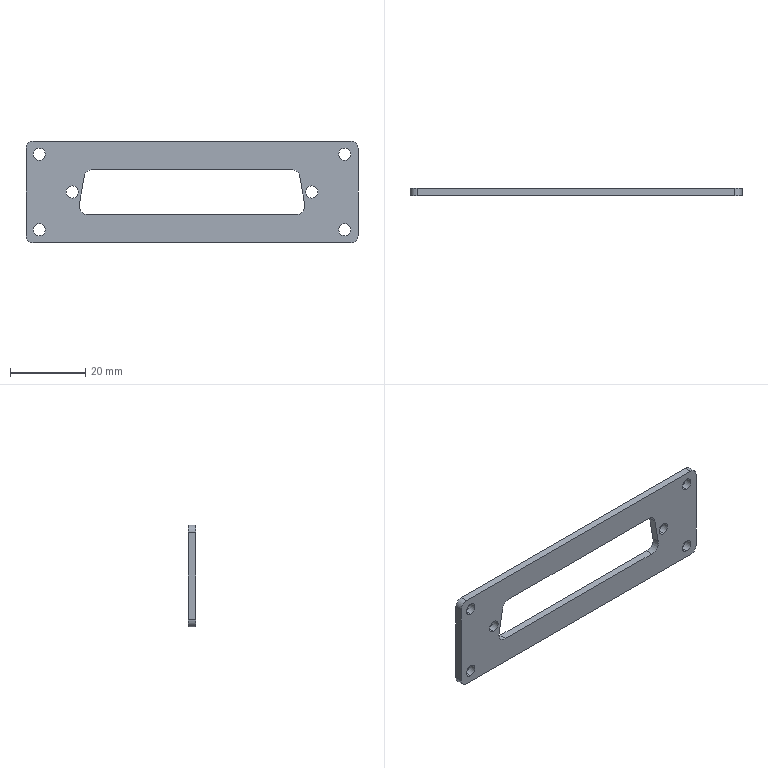Part | SolidWorks | features ICE 3, Extrusion 1, Fillet 1, HoleWzd 1 | 1 solid | 30 faces | box 88 x 2 x 27 mm | volume 3241 mm3 | cylinder 20 | plane 10 | commonest cylinder face diameters 3.2 x12 4 x4 4.8 x4
STEP:
#1=CARTESIAN_POINT('',(-31.75,0.,-1.6));
#2=VERTEX_POINT('',#1);
#3=CARTESIAN_POINT('',(-31.75,0.,1.6));
#4=VERTEX_POINT('',#3);
#5=CARTESIAN_POINT('',(-31.75,0.,0.));
#6=DIRECTION('',(0.,1.,0.));
#7=DIRECTION('',(0.,0.,1.));
#8=AXIS2_PLACEMENT_3D('',#5,#6,#7);
#9=CIRCLE('',#8,1.6);
#10=EDGE_CURVE('',#2,#4,#9,.T.);
#11=ORIENTED_EDGE('',*,*,#10,.F.);
#12=CARTESIAN_POINT('',(-31.75,2.,-1.6));
#13=VERTEX_POINT('',#12);
#14=CARTESIAN_POINT('',(-31.75,0.,-1.6));
#15=DIRECTION('',(0.,1.,0.));
#16=VECTOR('',#15,1000.);
#17=LINE('',#14,#16);
#18=EDGE_CURVE('',#2,#13,#17,.T.);
#19=ORIENTED_EDGE('',*,*,#18,.T.);
#20=CARTESIAN_POINT('',(-31.75,2.,1.6));
#21=VERTEX_POINT('',#20);
#22=CARTESIAN_POINT('',(-31.75,2.,0.));
#23=DIRECTION('',(0.,1.,0.));
#24=DIRECTION('',(0.,0.,1.));
#25=AXIS2_PLACEMENT_3D('',#22,#23,#24);
#26=CIRCLE('',#25,1.6);
#27=EDGE_CURVE('',#13,#21,#26,.T.);
#28=ORIENTED_EDGE('',*,*,#27,.T.);
#29=CARTESIAN_POINT('',(-31.75,0.,1.6));
#30=DIRECTION('',(0.,1.,0.));
#31=VECTOR('',#30,1000.);
#32=LINE('',#29,#31);
#33=EDGE_CURVE('',#4,#21,#32,.T.);
#34=ORIENTED_EDGE('',*,*,#33,.F.);
#35=EDGE_LOOP('',(#11,#19,#28,#34));
#36=FACE_OUTER_BOUND('',#35,.T.);
#37=CARTESIAN_POINT('',(-31.75,0.,0.));
#38=DIRECTION('',(0.,1.,0.));
#39=DIRECTION('',(0.,0.,1.));
#40=AXIS2_PLACEMENT_3D('',#37,#38,#39);
#41=CYLINDRICAL_SURFACE('',#40,1.6);
#42=ADVANCED_FACE('',(#36),#41,.F.);
#43=CARTESIAN_POINT('',(31.75,0.,-1.6));
#44=VERTEX_POINT('',#43);
#45=CARTESIAN_POINT('',(31.75,0.,1.6));
#46=VERTEX_POINT('',#45);
#47=CARTESIAN_POINT('',(31.75,0.,0.));
#48=DIRECTION('',(0.,1.,0.));
#49=DIRECTION('',(0.,0.,1.));
#50=AXIS2_PLACEMENT_3D('',#47,#48,#49);
#51=CIRCLE('',#50,1.6);
#52=EDGE_CURVE('',#44,#46,#51,.T.);
#53=ORIENTED_EDGE('',*,*,#52,.F.);
#54=CARTESIAN_POINT('',(31.75,2.,-1.6));
#55=VERTEX_POINT('',#54);
#56=CARTESIAN_POINT('',(31.75,0.,-1.6));
#57=DIRECTION('',(0.,1.,0.));
#58=VECTOR('',#57,1000.);
#59=LINE('',#56,#58);
#60=EDGE_CURVE('',#44,#55,#59,.T.);
#61=ORIENTED_EDGE('',*,*,#60,.T.);
#62=CARTESIAN_POINT('',(31.75,2.,1.6));
#63=VERTEX_POINT('',#62);
#64=CARTESIAN_POINT('',(31.75,2.,0.));
#65=DIRECTION('',(0.,1.,0.));
#66=DIRECTION('',(0.,0.,1.));
#67=AXIS2_PLACEMENT_3D('',#64,#65,#66);
#68=CIRCLE('',#67,1.6);
#69=EDGE_CURVE('',#55,#63,#68,.T.);
#70=ORIENTED_EDGE('',*,*,#69,.T.);
#71=CARTESIAN_POINT('',(31.75,0.,1.6));
#72=DIRECTION('',(0.,1.,0.));
#73=VECTOR('',#72,1000.);
#74=LINE('',#71,#73);
#75=EDGE_CURVE('',#46,#63,#74,.T.);
#76=ORIENTED_EDGE('',*,*,#75,.F.);
#77=EDGE_LOOP('',(#53,#61,#70,#76));
#78=FACE_OUTER_BOUND('',#77,.T.);
#79=CARTESIAN_POINT('',(31.75,0.,0.));
#80=DIRECTION('',(0.,1.,0.));
#81=DIRECTION('',(0.,0.,1.));
#82=AXIS2_PLACEMENT_3D('',#79,#80,#81);
#83=CYLINDRICAL_SURFACE('',#82,1.6);
#84=ADVANCED_FACE('',(#78),#83,.F.);
#85=CARTESIAN_POINT('',(-40.5,0.,8.4));
#86=VERTEX_POINT('',#85);
#87=CARTESIAN_POINT('',(-40.5,0.,11.6));
#88=VERTEX_POINT('',#87);
#89=CARTESIAN_POINT('',(-40.5,0.,10.));
#90=DIRECTION('',(0.,1.,0.));
#91=DIRECTION('',(0.,0.,1.));
#92=AXIS2_PLACEMENT_3D('',#89,#90,#91);
#93=CIRCLE('',#92,1.6);
#94=EDGE_CURVE('',#86,#88,#93,.T.);
#95=ORIENTED_EDGE('',*,*,#94,.F.);
#96=CARTESIAN_POINT('',(-40.5,2.,8.4));
#97=VERTEX_POINT('',#96);
#98=CARTESIAN_POINT('',(-40.5,0.,8.4));
#99=DIRECTION('',(0.,1.,0.));
#100=VECTOR('',#99,1000.);
#101=LINE('',#98,#100);
#102=EDGE_CURVE('',#86,#97,#101,.T.);
#103=ORIENTED_EDGE('',*,*,#102,.T.);
#104=CARTESIAN_POINT('',(-40.5,2.,11.6));
#105=VERTEX_POINT('',#104);
#106=CARTESIAN_POINT('',(-40.5,2.,10.));
#107=DIRECTION('',(0.,1.,0.));
#108=DIRECTION('',(0.,0.,1.));
#109=AXIS2_PLACEMENT_3D('',#106,#107,#108);
#110=CIRCLE('',#109,1.6);
#111=EDGE_CURVE('',#97,#105,#110,.T.);
#112=ORIENTED_EDGE('',*,*,#111,.T.);
#113=CARTESIAN_POINT('',(-40.5,0.,11.6));
#114=DIRECTION('',(0.,1.,0.));
#115=VECTOR('',#114,1000.);
#116=LINE('',#113,#115);
#117=EDGE_CURVE('',#88,#105,#116,.T.);
#118=ORIENTED_EDGE('',*,*,#117,.F.);
#119=EDGE_LOOP('',(#95,#103,#112,#118));
#120=FACE_OUTER_BOUND('',#119,.T.);
#121=CARTESIAN_POINT('',(-40.5,0.,10.));
#122=DIRECTION('',(0.,1.,0.));
#123=DIRECTION('',(0.,0.,1.));
#124=AXIS2_PLACEMENT_3D('',#121,#122,#123);
#125=CYLINDRICAL_SURFACE('',#124,1.6);
#126=ADVANCED_FACE('',(#120),#125,.F.);
#127=CARTESIAN_POINT('',(40.5,0.,8.4));
#128=VERTEX_POINT('',#127);
#129=CARTESIAN_POINT('',(40.5,0.,11.6));
#130=VERTEX_POINT('',#129);
#131=CARTESIAN_POINT('',(40.5,0.,10.));
#132=DIRECTION('',(0.,1.,0.));
#133=DIRECTION('',(0.,0.,1.));
#134=AXIS2_PLACEMENT_3D('',#131,#132,#133);
#135=CIRCLE('',#134,1.6);
#136=EDGE_CURVE('',#128,#130,#135,.T.);
#137=ORIENTED_EDGE('',*,*,#136,.F.);
#138=CARTESIAN_POINT('',(40.5,2.,8.4));
#139=VERTEX_POINT('',#138);
#140=CARTESIAN_POINT('',(40.5,0.,8.4));
#141=DIRECTION('',(0.,1.,0.));
#142=VECTOR('',#141,1000.);
#143=LINE('',#140,#142);
#144=EDGE_CURVE('',#128,#139,#143,.T.);
#145=ORIENTED_EDGE('',*,*,#144,.T.);
#146=CARTESIAN_POINT('',(40.5,2.,11.6));
#147=VERTEX_POINT('',#146);
#148=CARTESIAN_POINT('',(40.5,2.,10.));
#149=DIRECTION('',(0.,1.,0.));
#150=DIRECTION('',(0.,0.,1.));
#151=AXIS2_PLACEMENT_3D('',#148,#149,#150);
#152=CIRCLE('',#151,1.6);
#153=EDGE_CURVE('',#139,#147,#152,.T.);
#154=ORIENTED_EDGE('',*,*,#153,.T.);
#155=CARTESIAN_POINT('',(40.5,0.,11.6));
#156=DIRECTION('',(0.,1.,0.));
#157=VECTOR('',#156,1000.);
#158=LINE('',#155,#157);
#159=EDGE_CURVE('',#130,#147,#158,.T.);
#160=ORIENTED_EDGE('',*,*,#159,.F.);
#161=EDGE_LOOP('',(#137,#145,#154,#160));
#162=FACE_OUTER_BOUND('',#161,.T.);
#163=CARTESIAN_POINT('',(40.5,0.,10.));
#164=DIRECTION('',(0.,1.,0.));
#165=DIRECTION('',(0.,0.,1.));
#166=AXIS2_PLACEMENT_3D('',#163,#164,#165);
#167=CYLINDRICAL_SURFACE('',#166,1.6);
#168=ADVANCED_FACE('',(#162),#167,.F.);
#169=CARTESIAN_POINT('',(40.5,0.,-11.6));
#170=VERTEX_POINT('',#169);
#171=CARTESIAN_POINT('',(40.5,0.,-8.4));
#172=VERTEX_POINT('',#171);
#173=CARTESIAN_POINT('',(40.5,0.,-10.));
#174=DIRECTION('',(0.,1.,0.));
#175=DIRECTION('',(0.,0.,1.));
#176=AXIS2_PLACEMENT_3D('',#173,#174,#175);
#177=CIRCLE('',#176,1.6);
#178=EDGE_CURVE('',#170,#172,#177,.T.);
#179=ORIENTED_EDGE('',*,*,#178,.F.);
#180=CARTESIAN_POINT('',(40.5,2.,-11.6));
#181=VERTEX_POINT('',#180);
#182=CARTESIAN_POINT('',(40.5,0.,-11.6));
#183=DIRECTION('',(0.,1.,0.));
#184=VECTOR('',#183,1000.);
#185=LINE('',#182,#184);
#186=EDGE_CURVE('',#170,#181,#185,.T.);
#187=ORIENTED_EDGE('',*,*,#186,.T.);
#188=CARTESIAN_POINT('',(40.5,2.,-8.4));
#189=VERTEX_POINT('',#188);
#190=CARTESIAN_POINT('',(40.5,2.,-10.));
#191=DIRECTION('',(0.,1.,0.));
#192=DIRECTION('',(0.,0.,1.));
#193=AXIS2_PLACEMENT_3D('',#190,#191,#192);
#194=CIRCLE('',#193,1.6);
#195=EDGE_CURVE('',#181,#189,#194,.T.);
#196=ORIENTED_EDGE('',*,*,#195,.T.);
#197=CARTESIAN_POINT('',(40.5,0.,-8.4));
#198=DIRECTION('',(0.,1.,0.));
#199=VECTOR('',#198,1000.);
#200=LINE('',#197,#199);
#201=EDGE_CURVE('',#172,#189,#200,.T.);
#202=ORIENTED_EDGE('',*,*,#201,.F.);
#203=EDGE_LOOP('',(#179,#187,#196,#202));
#204=FACE_OUTER_BOUND('',#203,.T.);
#205=CARTESIAN_POINT('',(40.5,0.,-10.));
#206=DIRECTION('',(0.,1.,0.));
#207=DIRECTION('',(0.,0.,1.));
#208=AXIS2_PLACEMENT_3D('',#205,#206,#207);
#209=CYLINDRICAL_SURFACE('',#208,1.6);
#210=ADVANCED_FACE('',(#204),#209,.F.);
#211=CARTESIAN_POINT('',(-40.5,0.,-11.6));
#212=VERTEX_POINT('',#211);
#213=CARTESIAN_POINT('',(-40.5,0.,-8.4));
#214=VERTEX_POINT('',#213);
#215=CARTESIAN_POINT('',(-40.5,0.,-10.));
#216=DIRECTION('',(0.,1.,0.));
#217=DIRECTION('',(0.,0.,1.));
#218=AXIS2_PLACEMENT_3D('',#215,#216,#217);
#219=CIRCLE('',#218,1.6);
#220=EDGE_CURVE('',#212,#214,#219,.T.);
#221=ORIENTED_EDGE('',*,*,#220,.F.);
#222=CARTESIAN_POINT('',(-40.5,2.,-11.6));
#223=VERTEX_POINT('',#222);
#224=CARTESIAN_POINT('',(-40.5,0.,-11.6));
#225=DIRECTION('',(0.,1.,0.));
#226=VECTOR('',#225,1000.);
#227=LINE('',#224,#226);
#228=EDGE_CURVE('',#212,#223,#227,.T.);
#229=ORIENTED_EDGE('',*,*,#228,.T.);
#230=CARTESIAN_POINT('',(-40.5,2.,-8.4));
#231=VERTEX_POINT('',#230);
#232=CARTESIAN_POINT('',(-40.5,2.,-10.));
#233=DIRECTION('',(0.,1.,0.));
#234=DIRECTION('',(0.,0.,1.));
#235=AXIS2_PLACEMENT_3D('',#232,#233,#234);
#236=CIRCLE('',#235,1.6);
#237=EDGE_CURVE('',#223,#231,#236,.T.);
#238=ORIENTED_EDGE('',*,*,#237,.T.);
#239=CARTESIAN_POINT('',(-40.5,0.,-8.4));
#240=DIRECTION('',(0.,1.,0.));
#241=VECTOR('',#240,1000.);
#242=LINE('',#239,#241);
#243=EDGE_CURVE('',#214,#231,#242,.T.);
#244=ORIENTED_EDGE('',*,*,#243,.F.);
#245=EDGE_LOOP('',(#221,#229,#238,#244));
#246=FACE_OUTER_BOUND('',#245,.T.);
#247=CARTESIAN_POINT('',(-40.5,0.,-10.));
#248=DIRECTION('',(0.,1.,0.));
#249=DIRECTION('',(0.,0.,1.));
#250=AXIS2_PLACEMENT_3D('',#247,#248,#249);
#251=CYLINDRICAL_SURFACE('',#250,1.6);
#252=ADVANCED_FACE('',(#246),#251,.F.);
#253=CARTESIAN_POINT('',(-31.75,2.,0.));
#254=DIRECTION('',(0.,1.,0.));
#255=DIRECTION('',(0.,0.,1.));
#256=AXIS2_PLACEMENT_3D('',#253,#254,#255);
#257=CIRCLE('',#256,1.6);
#258=EDGE_CURVE('',#21,#13,#257,.T.);
#259=ORIENTED_EDGE('',*,*,#258,.F.);
#260=ORIENTED_EDGE('',*,*,#27,.F.);
#261=EDGE_LOOP('',(#259,#260));
#262=FACE_BOUND('',#261,.T.);
#263=CARTESIAN_POINT('',(31.75,2.,0.));
#264=DIRECTION('',(0.,1.,0.));
#265=DIRECTION('',(0.,0.,1.));
#266=AXIS2_PLACEMENT_3D('',#263,#264,#265);
#267=CIRCLE('',#266,1.6);
#268=EDGE_CURVE('',#63,#55,#267,.T.);
#269=ORIENTED_EDGE('',*,*,#268,.F.);
#270=ORIENTED_EDGE('',*,*,#69,.F.);
#271=EDGE_LOOP('',(#269,#270));
#272=FACE_BOUND('',#271,.T.);
#273=CARTESIAN_POINT('',(-29.864,2.,-3.233));
#274=VERTEX_POINT('',#273);
#275=CARTESIAN_POINT('',(-28.576,2.,4.067));
#276=VERTEX_POINT('',#275);
#277=CARTESIAN_POINT('',(-29.864,2.,-3.233));
#278=DIRECTION('',(0.1736,0.,0.9848));
#279=VECTOR('',#278,1000.);
#280=LINE('',#277,#279);
#281=EDGE_CURVE('',#274,#276,#280,.T.);
#282=ORIENTED_EDGE('',*,*,#281,.F.);
#283=CARTESIAN_POINT('',(-27.5,2.,-6.05));
#284=VERTEX_POINT('',#283);
#285=CARTESIAN_POINT('',(-27.5,2.,-3.65));
#286=DIRECTION('',(0.,1.,0.));
#287=DIRECTION('',(0.,0.,-1.));
#288=AXIS2_PLACEMENT_3D('',#285,#286,#287);
#289=CIRCLE('',#288,2.4);
#290=EDGE_CURVE('',#284,#274,#289,.T.);
#291=ORIENTED_EDGE('',*,*,#290,.F.);
#292=CARTESIAN_POINT('',(27.5,2.,-6.05));
#293=VERTEX_POINT('',#292);
#294=CARTESIAN_POINT('',(-27.5,2.,-6.05));
#295=DIRECTION('',(-1.,0.,0.));
#296=VECTOR('',#295,1000.);
#297=LINE('',#294,#296);
#298=EDGE_CURVE('',#293,#284,#297,.T.);
#299=ORIENTED_EDGE('',*,*,#298,.F.);
#300=CARTESIAN_POINT('',(29.864,2.,-3.233));
#301=VERTEX_POINT('',#300);
#302=CARTESIAN_POINT('',(27.5,2.,-3.65));
#303=DIRECTION('',(0.,1.,0.));
#304=DIRECTION('',(0.,0.,-1.));
#305=AXIS2_PLACEMENT_3D('',#302,#303,#304);
#306=CIRCLE('',#305,2.4);
#307=EDGE_CURVE('',#301,#293,#306,.T.);
#308=ORIENTED_EDGE('',*,*,#307,.F.);
#309=CARTESIAN_POINT('',(28.576,2.,4.067));
#310=VERTEX_POINT('',#309);
#311=CARTESIAN_POINT('',(29.864,2.,-3.233));
#312=DIRECTION('',(0.1736,0.,-0.9848));
#313=VECTOR('',#312,1000.);
#314=LINE('',#311,#313);
#315=EDGE_CURVE('',#310,#301,#314,.T.);
#316=ORIENTED_EDGE('',*,*,#315,.F.);
#317=CARTESIAN_POINT('',(26.213,2.,6.05));
#318=VERTEX_POINT('',#317);
#319=CARTESIAN_POINT('',(26.213,2.,3.65));
#320=DIRECTION('',(0.,1.,0.));
#321=DIRECTION('',(0.,0.,-1.));
#322=AXIS2_PLACEMENT_3D('',#319,#320,#321);
#323=CIRCLE('',#322,2.4);
#324=EDGE_CURVE('',#318,#310,#323,.T.);
#325=ORIENTED_EDGE('',*,*,#324,.F.);
#326=CARTESIAN_POINT('',(-26.213,2.,6.05));
#327=VERTEX_POINT('',#326);
#328=CARTESIAN_POINT('',(-26.213,2.,6.05));
#329=DIRECTION('',(1.,0.,0.));
#330=VECTOR('',#329,1000.);
#331=LINE('',#328,#330);
#332=EDGE_CURVE('',#327,#318,#331,.T.);
#333=ORIENTED_EDGE('',*,*,#332,.F.);
#334=CARTESIAN_POINT('',(-26.213,2.,3.65));
#335=DIRECTION('',(0.,1.,0.));
#336=DIRECTION('',(0.,0.,1.));
#337=AXIS2_PLACEMENT_3D('',#334,#335,#336);
#338=CIRCLE('',#337,2.4);
#339=EDGE_CURVE('',#276,#327,#338,.T.);
#340=ORIENTED_EDGE('',*,*,#339,.F.);
#341=EDGE_LOOP('',(#282,#291,#299,#308,#316,#325,#333,#340));
#342=FACE_BOUND('',#341,.T.);
#343=CARTESIAN_POINT('',(-40.5,2.,10.));
#344=DIRECTION('',(0.,1.,0.));
#345=DIRECTION('',(0.,0.,1.));
#346=AXIS2_PLACEMENT_3D('',#343,#344,#345);
#347=CIRCLE('',#346,1.6);
#348=EDGE_CURVE('',#105,#97,#347,.T.);
#349=ORIENTED_EDGE('',*,*,#348,.F.);
#350=ORIENTED_EDGE('',*,*,#111,.F.);
#351=EDGE_LOOP('',(#349,#350));
#352=FACE_BOUND('',#351,.T.);
#353=CARTESIAN_POINT('',(40.5,2.,10.));
#354=DIRECTION('',(0.,1.,0.));
#355=DIRECTION('',(0.,0.,1.));
#356=AXIS2_PLACEMENT_3D('',#353,#354,#355);
#357=CIRCLE('',#356,1.6);
#358=EDGE_CURVE('',#147,#139,#357,.T.);
#359=ORIENTED_EDGE('',*,*,#358,.F.);
#360=ORIENTED_EDGE('',*,*,#153,.F.);
#361=EDGE_LOOP('',(#359,#360));
#362=FACE_BOUND('',#361,.T.);
#363=CARTESIAN_POINT('',(40.5,2.,-10.));
#364=DIRECTION('',(0.,1.,0.));
#365=DIRECTION('',(0.,0.,1.));
#366=AXIS2_PLACEMENT_3D('',#363,#364,#365);
#367=CIRCLE('',#366,1.6);
#368=EDGE_CURVE('',#189,#181,#367,.T.);
#369=ORIENTED_EDGE('',*,*,#368,.F.);
#370=ORIENTED_EDGE('',*,*,#195,.F.);
#371=EDGE_LOOP('',(#369,#370));
#372=FACE_BOUND('',#371,.T.);
#373=CARTESIAN_POINT('',(-40.5,2.,-10.));
#374=DIRECTION('',(0.,1.,0.));
#375=DIRECTION('',(0.,0.,1.));
#376=AXIS2_PLACEMENT_3D('',#373,#374,#375);
#377=CIRCLE('',#376,1.6);
#378=EDGE_CURVE('',#231,#223,#377,.T.);
#379=ORIENTED_EDGE('',*,*,#378,.F.);
#380=ORIENTED_EDGE('',*,*,#237,.F.);
#381=EDGE_LOOP('',(#379,#380));
#382=FACE_BOUND('',#381,.T.);
#383=CARTESIAN_POINT('',(44.,2.,11.5));
#384=VERTEX_POINT('',#383);
#385=CARTESIAN_POINT('',(44.,2.,-11.5));
#386=VERTEX_POINT('',#385);
#387=CARTESIAN_POINT('',(44.,2.,13.5));
#388=DIRECTION('',(0.,0.,-1.));
#389=VECTOR('',#388,1000.);
#390=LINE('',#387,#389);
#391=EDGE_CURVE('',#384,#386,#390,.T.);
#392=ORIENTED_EDGE('',*,*,#391,.T.);
#393=CARTESIAN_POINT('',(42.,2.,-13.5));
#394=VERTEX_POINT('',#393);
#395=CARTESIAN_POINT('',(42.,2.,-11.5));
#396=DIRECTION('',(0.,1.,0.));
#397=DIRECTION('',(0.,0.,-1.));
#398=AXIS2_PLACEMENT_3D('',#395,#396,#397);
#399=CIRCLE('',#398,2.);
#400=EDGE_CURVE('',#386,#394,#399,.T.);
#401=ORIENTED_EDGE('',*,*,#400,.T.);
#402=CARTESIAN_POINT('',(-42.,2.,-13.5));
#403=VERTEX_POINT('',#402);
#404=CARTESIAN_POINT('',(-44.,2.,-13.5));
#405=DIRECTION('',(-1.,0.,0.));
#406=VECTOR('',#405,1000.);
#407=LINE('',#404,#406);
#408=EDGE_CURVE('',#394,#403,#407,.T.);
#409=ORIENTED_EDGE('',*,*,#408,.T.);
#410=CARTESIAN_POINT('',(-44.,2.,-11.5));
#411=VERTEX_POINT('',#410);
#412=CARTESIAN_POINT('',(-42.,2.,-11.5));
#413=DIRECTION('',(0.,1.,0.));
#414=DIRECTION('',(0.,0.,-1.));
#415=AXIS2_PLACEMENT_3D('',#412,#413,#414);
#416=CIRCLE('',#415,2.);
#417=EDGE_CURVE('',#403,#411,#416,.T.);
#418=ORIENTED_EDGE('',*,*,#417,.T.);
#419=CARTESIAN_POINT('',(-44.,2.,11.5));
#420=VERTEX_POINT('',#419);
#421=CARTESIAN_POINT('',(-44.,2.,13.5));
#422=DIRECTION('',(0.,0.,1.));
#423=VECTOR('',#422,1000.);
#424=LINE('',#421,#423);
#425=EDGE_CURVE('',#411,#420,#424,.T.);
#426=ORIENTED_EDGE('',*,*,#425,.T.);
#427=CARTESIAN_POINT('',(-42.,2.,13.5));
#428=VERTEX_POINT('',#427);
#429=CARTESIAN_POINT('',(-42.,2.,11.5));
#430=DIRECTION('',(0.,1.,0.));
#431=DIRECTION('',(0.,0.,-1.));
#432=AXIS2_PLACEMENT_3D('',#429,#430,#431);
#433=CIRCLE('',#432,2.);
#434=EDGE_CURVE('',#420,#428,#433,.T.);
#435=ORIENTED_EDGE('',*,*,#434,.T.);
#436=CARTESIAN_POINT('',(42.,2.,13.5));
#437=VERTEX_POINT('',#436);
#438=CARTESIAN_POINT('',(-44.,2.,13.5));
#439=DIRECTION('',(1.,0.,0.));
#440=VECTOR('',#439,1000.);
#441=LINE('',#438,#440);
#442=EDGE_CURVE('',#428,#437,#441,.T.);
#443=ORIENTED_EDGE('',*,*,#442,.T.);
#444=CARTESIAN_POINT('',(42.,2.,11.5));
#445=DIRECTION('',(0.,1.,0.));
#446=DIRECTION('',(0.,0.,-1.));
#447=AXIS2_PLACEMENT_3D('',#444,#445,#446);
#448=CIRCLE('',#447,2.);
#449=EDGE_CURVE('',#437,#384,#448,.T.);
#450=ORIENTED_EDGE('',*,*,#449,.T.);
#451=EDGE_LOOP('',(#392,#401,#409,#418,#426,#435,#443,#450));
#452=FACE_OUTER_BOUND('',#451,.T.);
#453=CARTESIAN_POINT('',(0.,2.,0.));
#454=DIRECTION('',(0.,-1.,0.));
#455=DIRECTION('',(0.,0.,-1.));
#456=AXIS2_PLACEMENT_3D('',#453,#454,#455);
#457=PLANE('',#456);
#458=ADVANCED_FACE('',(#262,#272,#342,#352,#362,#372,#382,#452),#457,.F.);
#459=CARTESIAN_POINT('',(44.,0.,11.5));
#460=VERTEX_POINT('',#459);
#461=CARTESIAN_POINT('',(44.,0.,-11.5));
#462=VERTEX_POINT('',#461);
#463=CARTESIAN_POINT('',(44.,0.,13.5));
#464=DIRECTION('',(0.,0.,-1.));
#465=VECTOR('',#464,1000.);
#466=LINE('',#463,#465);
#467=EDGE_CURVE('',#460,#462,#466,.T.);
#468=ORIENTED_EDGE('',*,*,#467,.T.);
#469=CARTESIAN_POINT('',(44.,2.,-11.5));
#470=DIRECTION('',(0.,1.,0.));
#471=VECTOR('',#470,1000.);
#472=LINE('',#469,#471);
#473=EDGE_CURVE('',#462,#386,#472,.T.);
#474=ORIENTED_EDGE('',*,*,#473,.T.);
#475=ORIENTED_EDGE('',*,*,#391,.F.);
#476=CARTESIAN_POINT('',(44.,2.,11.5));
#477=DIRECTION('',(0.,-1.,0.));
#478=VECTOR('',#477,1000.);
#479=LINE('',#476,#478);
#480=EDGE_CURVE('',#384,#460,#479,.T.);
#481=ORIENTED_EDGE('',*,*,#480,.T.);
#482=EDGE_LOOP('',(#468,#474,#475,#481));
#483=FACE_OUTER_BOUND('',#482,.T.);
#484=CARTESIAN_POINT('',(44.,2.,13.5));
#485=DIRECTION('',(-1.,0.,0.));
#486=DIRECTION('',(0.,0.,1.));
#487=AXIS2_PLACEMENT_3D('',#484,#485,#486);
#488=PLANE('',#487);
#489=ADVANCED_FACE('',(#483),#488,.F.);
#490=ORIENTED_EDGE('',*,*,#408,.F.);
#491=CARTESIAN_POINT('',(42.,0.,-13.5));
#492=VERTEX_POINT('',#491);
#493=CARTESIAN_POINT('',(42.,2.,-13.5));
#494=DIRECTION('',(0.,-1.,0.));
#495=VECTOR('',#494,1000.);
#496=LINE('',#493,#495);
#497=EDGE_CURVE('',#394,#492,#496,.T.);
#498=ORIENTED_EDGE('',*,*,#497,.T.);
#499=CARTESIAN_POINT('',(-42.,0.,-13.5));
#500=VERTEX_POINT('',#499);
#501=CARTESIAN_POINT('',(-44.,0.,-13.5));
#502=DIRECTION('',(-1.,0.,0.));
#503=VECTOR('',#502,1000.);
#504=LINE('',#501,#503);
#505=EDGE_CURVE('',#492,#500,#504,.T.);
#506=ORIENTED_EDGE('',*,*,#505,.T.);
#507=CARTESIAN_POINT('',(-42.,2.,-13.5));
#508=DIRECTION('',(0.,1.,0.));
#509=VECTOR('',#508,1000.);
#510=LINE('',#507,#509);
#511=EDGE_CURVE('',#500,#403,#510,.T.);
#512=ORIENTED_EDGE('',*,*,#511,.T.);
#513=EDGE_LOOP('',(#490,#498,#506,#512));
#514=FACE_OUTER_BOUND('',#513,.T.);
#515=CARTESIAN_POINT('',(-44.,2.,-13.5));
#516=DIRECTION('',(0.,0.,1.));
#517=DIRECTION('',(1.,0.,0.));
#518=AXIS2_PLACEMENT_3D('',#515,#516,#517);
#519=PLANE('',#518);
#520=ADVANCED_FACE('',(#514),#519,.F.);
#521=CARTESIAN_POINT('',(-44.,0.,-11.5));
#522=VERTEX_POINT('',#521);
#523=CARTESIAN_POINT('',(-44.,0.,11.5));
#524=VERTEX_POINT('',#523);
#525=CARTESIAN_POINT('',(-44.,0.,13.5));
#526=DIRECTION('',(0.,0.,1.));
#527=VECTOR('',#526,1000.);
#528=LINE('',#525,#527);
#529=EDGE_CURVE('',#522,#524,#528,.T.);
#530=ORIENTED_EDGE('',*,*,#529,.T.);
#531=CARTESIAN_POINT('',(-44.,2.,11.5));
#532=DIRECTION('',(0.,1.,0.));
#533=VECTOR('',#532,1000.);
#534=LINE('',#531,#533);
#535=EDGE_CURVE('',#524,#420,#534,.T.);
#536=ORIENTED_EDGE('',*,*,#535,.T.);
#537=ORIENTED_EDGE('',*,*,#425,.F.);
#538=CARTESIAN_POINT('',(-44.,2.,-11.5));
#539=DIRECTION('',(0.,-1.,0.));
#540=VECTOR('',#539,1000.);
#541=LINE('',#538,#540);
#542=EDGE_CURVE('',#411,#522,#541,.T.);
#543=ORIENTED_EDGE('',*,*,#542,.T.);
#544=EDGE_LOOP('',(#530,#536,#537,#543));
#545=FACE_OUTER_BOUND('',#544,.T.);
#546=CARTESIAN_POINT('',(-44.,2.,13.5));
#547=DIRECTION('',(1.,0.,0.));
#548=DIRECTION('',(0.,0.,-1.));
#549=AXIS2_PLACEMENT_3D('',#546,#547,#548);
#550=PLANE('',#549);
#551=ADVANCED_FACE('',(#545),#550,.F.);
#552=CARTESIAN_POINT('',(-42.,0.,13.5));
#553=VERTEX_POINT('',#552);
#554=CARTESIAN_POINT('',(42.,0.,13.5));
#555=VERTEX_POINT('',#554);
#556=CARTESIAN_POINT('',(-44.,0.,13.5));
#557=DIRECTION('',(1.,0.,0.));
#558=VECTOR('',#557,1000.);
#559=LINE('',#556,#558);
#560=EDGE_CURVE('',#553,#555,#559,.T.);
#561=ORIENTED_EDGE('',*,*,#560,.T.);
#562=CARTESIAN_POINT('',(42.,2.,13.5));
#563=DIRECTION('',(0.,1.,0.));
#564=VECTOR('',#563,1000.);
#565=LINE('',#562,#564);
#566=EDGE_CURVE('',#555,#437,#565,.T.);
#567=ORIENTED_EDGE('',*,*,#566,.T.);
#568=ORIENTED_EDGE('',*,*,#442,.F.);
#569=CARTESIAN_POINT('',(-42.,2.,13.5));
#570=DIRECTION('',(0.,-1.,0.));
#571=VECTOR('',#570,1000.);
#572=LINE('',#569,#571);
#573=EDGE_CURVE('',#428,#553,#572,.T.);
#574=ORIENTED_EDGE('',*,*,#573,.T.);
#575=EDGE_LOOP('',(#561,#567,#568,#574));
#576=FACE_OUTER_BOUND('',#575,.T.);
#577=CARTESIAN_POINT('',(-44.,2.,13.5));
#578=DIRECTION('',(0.,0.,-1.));
#579=DIRECTION('',(-1.,0.,0.));
#580=AXIS2_PLACEMENT_3D('',#577,#578,#579);
#581=PLANE('',#580);
#582=ADVANCED_FACE('',(#576),#581,.F.);
#583=CARTESIAN_POINT('',(-31.75,0.,0.));
#584=DIRECTION('',(0.,1.,0.));
#585=DIRECTION('',(0.,0.,1.));
#586=AXIS2_PLACEMENT_3D('',#583,#584,#585);
#587=CIRCLE('',#586,1.6);
#588=EDGE_CURVE('',#4,#2,#587,.T.);
#589=ORIENTED_EDGE('',*,*,#588,.T.);
#590=ORIENTED_EDGE('',*,*,#10,.T.);
#591=EDGE_LOOP('',(#589,#590));
#592=FACE_BOUND('',#591,.T.);
#593=CARTESIAN_POINT('',(31.75,0.,0.));
#594=DIRECTION('',(0.,1.,0.));
#595=DIRECTION('',(0.,0.,1.));
#596=AXIS2_PLACEMENT_3D('',#593,#594,#595);
#597=CIRCLE('',#596,1.6);
#598=EDGE_CURVE('',#46,#44,#597,.T.);
#599=ORIENTED_EDGE('',*,*,#598,.T.);
#600=ORIENTED_EDGE('',*,*,#52,.T.);
#601=EDGE_LOOP('',(#599,#600));
#602=FACE_BOUND('',#601,.T.);
#603=CARTESIAN_POINT('',(-27.5,0.,-6.05));
#604=VERTEX_POINT('',#603);
#605=CARTESIAN_POINT('',(-29.864,0.,-3.233));
#606=VERTEX_POINT('',#605);
#607=CARTESIAN_POINT('',(-27.5,0.,-3.65));
#608=DIRECTION('',(0.,1.,0.));
#609=DIRECTION('',(0.,0.,-1.));
#610=AXIS2_PLACEMENT_3D('',#607,#608,#609);
#611=CIRCLE('',#610,2.4);
#612=EDGE_CURVE('',#604,#606,#611,.T.);
#613=ORIENTED_EDGE('',*,*,#612,.T.);
#614=CARTESIAN_POINT('',(-28.576,0.,4.067));
#615=VERTEX_POINT('',#614);
#616=CARTESIAN_POINT('',(-29.864,0.,-3.233));
#617=DIRECTION('',(0.1736,0.,0.9848));
#618=VECTOR('',#617,1000.);
#619=LINE('',#616,#618);
#620=EDGE_CURVE('',#606,#615,#619,.T.);
#621=ORIENTED_EDGE('',*,*,#620,.T.);
#622=CARTESIAN_POINT('',(-26.213,0.,6.05));
#623=VERTEX_POINT('',#622);
#624=CARTESIAN_POINT('',(-26.213,0.,3.65));
#625=DIRECTION('',(0.,1.,0.));
#626=DIRECTION('',(0.,0.,1.));
#627=AXIS2_PLACEMENT_3D('',#624,#625,#626);
#628=CIRCLE('',#627,2.4);
#629=EDGE_CURVE('',#615,#623,#628,.T.);
#630=ORIENTED_EDGE('',*,*,#629,.T.);
#631=CARTESIAN_POINT('',(26.213,0.,6.05));
#632=VERTEX_POINT('',#631);
#633=CARTESIAN_POINT('',(-26.213,0.,6.05));
#634=DIRECTION('',(1.,0.,0.));
#635=VECTOR('',#634,1000.);
#636=LINE('',#633,#635);
#637=EDGE_CURVE('',#623,#632,#636,.T.);
#638=ORIENTED_EDGE('',*,*,#637,.T.);
#639=CARTESIAN_POINT('',(28.576,0.,4.067));
#640=VERTEX_POINT('',#639);
#641=CARTESIAN_POINT('',(26.213,0.,3.65));
#642=DIRECTION('',(0.,1.,0.));
#643=DIRECTION('',(0.,0.,-1.));
#644=AXIS2_PLACEMENT_3D('',#641,#642,#643);
#645=CIRCLE('',#644,2.4);
#646=EDGE_CURVE('',#632,#640,#645,.T.);
#647=ORIENTED_EDGE('',*,*,#646,.T.);
#648=CARTESIAN_POINT('',(29.864,0.,-3.233));
#649=VERTEX_POINT('',#648);
#650=CARTESIAN_POINT('',(29.864,0.,-3.233));
#651=DIRECTION('',(0.1736,0.,-0.9848));
#652=VECTOR('',#651,1000.);
#653=LINE('',#650,#652);
#654=EDGE_CURVE('',#640,#649,#653,.T.);
#655=ORIENTED_EDGE('',*,*,#654,.T.);
#656=CARTESIAN_POINT('',(27.5,0.,-6.05));
#657=VERTEX_POINT('',#656);
#658=CARTESIAN_POINT('',(27.5,0.,-3.65));
#659=DIRECTION('',(0.,1.,0.));
#660=DIRECTION('',(0.,0.,-1.));
#661=AXIS2_PLACEMENT_3D('',#658,#659,#660);
#662=CIRCLE('',#661,2.4);
#663=EDGE_CURVE('',#649,#657,#662,.T.);
#664=ORIENTED_EDGE('',*,*,#663,.T.);
#665=CARTESIAN_POINT('',(-27.5,0.,-6.05));
#666=DIRECTION('',(-1.,0.,0.));
#667=VECTOR('',#666,1000.);
#668=LINE('',#665,#667);
#669=EDGE_CURVE('',#657,#604,#668,.T.);
#670=ORIENTED_EDGE('',*,*,#669,.T.);
#671=EDGE_LOOP('',(#613,#621,#630,#638,#647,#655,#664,#670));
#672=FACE_BOUND('',#671,.T.);
#673=CARTESIAN_POINT('',(-40.5,0.,10.));
#674=DIRECTION('',(0.,1.,0.));
#675=DIRECTION('',(0.,0.,1.));
#676=AXIS2_PLACEMENT_3D('',#673,#674,#675);
#677=CIRCLE('',#676,1.6);
#678=EDGE_CURVE('',#88,#86,#677,.T.);
#679=ORIENTED_EDGE('',*,*,#678,.T.);
#680=ORIENTED_EDGE('',*,*,#94,.T.);
#681=EDGE_LOOP('',(#679,#680));
#682=FACE_BOUND('',#681,.T.);
#683=CARTESIAN_POINT('',(40.5,0.,10.));
#684=DIRECTION('',(0.,1.,0.));
#685=DIRECTION('',(0.,0.,1.));
#686=AXIS2_PLACEMENT_3D('',#683,#684,#685);
#687=CIRCLE('',#686,1.6);
#688=EDGE_CURVE('',#130,#128,#687,.T.);
#689=ORIENTED_EDGE('',*,*,#688,.T.);
#690=ORIENTED_EDGE('',*,*,#136,.T.);
#691=EDGE_LOOP('',(#689,#690));
#692=FACE_BOUND('',#691,.T.);
#693=CARTESIAN_POINT('',(40.5,0.,-10.));
#694=DIRECTION('',(0.,1.,0.));
#695=DIRECTION('',(0.,0.,1.));
#696=AXIS2_PLACEMENT_3D('',#693,#694,#695);
#697=CIRCLE('',#696,1.6);
#698=EDGE_CURVE('',#172,#170,#697,.T.);
#699=ORIENTED_EDGE('',*,*,#698,.T.);
#700=ORIENTED_EDGE('',*,*,#178,.T.);
#701=EDGE_LOOP('',(#699,#700));
#702=FACE_BOUND('',#701,.T.);
#703=CARTESIAN_POINT('',(-40.5,0.,-10.));
#704=DIRECTION('',(0.,1.,0.));
#705=DIRECTION('',(0.,0.,1.));
#706=AXIS2_PLACEMENT_3D('',#703,#704,#705);
#707=CIRCLE('',#706,1.6);
#708=EDGE_CURVE('',#214,#212,#707,.T.);
#709=ORIENTED_EDGE('',*,*,#708,.T.);
#710=ORIENTED_EDGE('',*,*,#220,.T.);
#711=EDGE_LOOP('',(#709,#710));
#712=FACE_BOUND('',#711,.T.);
#713=ORIENTED_EDGE('',*,*,#505,.F.);
#714=CARTESIAN_POINT('',(42.,0.,-11.5));
#715=DIRECTION('',(0.,-1.,0.));
#716=DIRECTION('',(0.,0.,-1.));
#717=AXIS2_PLACEMENT_3D('',#714,#715,#716);
#718=CIRCLE('',#717,2.);
#719=EDGE_CURVE('',#492,#462,#718,.T.);
#720=ORIENTED_EDGE('',*,*,#719,.T.);
#721=ORIENTED_EDGE('',*,*,#467,.F.);
#722=CARTESIAN_POINT('',(42.,0.,11.5));
#723=DIRECTION('',(0.,-1.,0.));
#724=DIRECTION('',(0.,0.,-1.));
#725=AXIS2_PLACEMENT_3D('',#722,#723,#724);
#726=CIRCLE('',#725,2.);
#727=EDGE_CURVE('',#460,#555,#726,.T.);
#728=ORIENTED_EDGE('',*,*,#727,.T.);
#729=ORIENTED_EDGE('',*,*,#560,.F.);
#730=CARTESIAN_POINT('',(-42.,0.,11.5));
#731=DIRECTION('',(0.,-1.,0.));
#732=DIRECTION('',(0.,0.,-1.));
#733=AXIS2_PLACEMENT_3D('',#730,#731,#732);
#734=CIRCLE('',#733,2.);
#735=EDGE_CURVE('',#553,#524,#734,.T.);
#736=ORIENTED_EDGE('',*,*,#735,.T.);
#737=ORIENTED_EDGE('',*,*,#529,.F.);
#738=CARTESIAN_POINT('',(-42.,0.,-11.5));
#739=DIRECTION('',(0.,-1.,0.));
#740=DIRECTION('',(0.,0.,-1.));
#741=AXIS2_PLACEMENT_3D('',#738,#739,#740);
#742=CIRCLE('',#741,2.);
#743=EDGE_CURVE('',#522,#500,#742,.T.);
#744=ORIENTED_EDGE('',*,*,#743,.T.);
#745=EDGE_LOOP('',(#713,#720,#721,#728,#729,#736,#737,#744));
#746=FACE_OUTER_BOUND('',#745,.T.);
#747=CARTESIAN_POINT('',(0.,0.,0.));
#748=DIRECTION('',(0.,-1.,0.));
#749=DIRECTION('',(0.,0.,-1.));
#750=AXIS2_PLACEMENT_3D('',#747,#748,#749);
#751=PLANE('',#750);
#752=ADVANCED_FACE('',(#592,#602,#672,#682,#692,#702,#712,#746),#751,.T.);
#753=ORIENTED_EDGE('',*,*,#228,.F.);
#754=ORIENTED_EDGE('',*,*,#708,.F.);
#755=ORIENTED_EDGE('',*,*,#243,.T.);
#756=ORIENTED_EDGE('',*,*,#378,.T.);
#757=EDGE_LOOP('',(#753,#754,#755,#756));
#758=FACE_OUTER_BOUND('',#757,.T.);
#759=CARTESIAN_POINT('',(-40.5,0.,-10.));
#760=DIRECTION('',(0.,1.,0.));
#761=DIRECTION('',(0.,0.,1.));
#762=AXIS2_PLACEMENT_3D('',#759,#760,#761);
#763=CYLINDRICAL_SURFACE('',#762,1.6);
#764=ADVANCED_FACE('',(#758),#763,.F.);
#765=ORIENTED_EDGE('',*,*,#186,.F.);
#766=ORIENTED_EDGE('',*,*,#698,.F.);
#767=ORIENTED_EDGE('',*,*,#201,.T.);
#768=ORIENTED_EDGE('',*,*,#368,.T.);
#769=EDGE_LOOP('',(#765,#766,#767,#768));
#770=FACE_OUTER_BOUND('',#769,.T.);
#771=CARTESIAN_POINT('',(40.5,0.,-10.));
#772=DIRECTION('',(0.,1.,0.));
#773=DIRECTION('',(0.,0.,1.));
#774=AXIS2_PLACEMENT_3D('',#771,#772,#773);
#775=CYLINDRICAL_SURFACE('',#774,1.6);
#776=ADVANCED_FACE('',(#770),#775,.F.);
#777=ORIENTED_EDGE('',*,*,#144,.F.);
#778=ORIENTED_EDGE('',*,*,#688,.F.);
#779=ORIENTED_EDGE('',*,*,#159,.T.);
#780=ORIENTED_EDGE('',*,*,#358,.T.);
#781=EDGE_LOOP('',(#777,#778,#779,#780));
#782=FACE_OUTER_BOUND('',#781,.T.);
#783=CARTESIAN_POINT('',(40.5,0.,10.));
#784=DIRECTION('',(0.,1.,0.));
#785=DIRECTION('',(0.,0.,1.));
#786=AXIS2_PLACEMENT_3D('',#783,#784,#785);
#787=CYLINDRICAL_SURFACE('',#786,1.6);
#788=ADVANCED_FACE('',(#782),#787,.F.);
#789=ORIENTED_EDGE('',*,*,#102,.F.);
#790=ORIENTED_EDGE('',*,*,#678,.F.);
#791=ORIENTED_EDGE('',*,*,#117,.T.);
#792=ORIENTED_EDGE('',*,*,#348,.T.);
#793=EDGE_LOOP('',(#789,#790,#791,#792));
#794=FACE_OUTER_BOUND('',#793,.T.);
#795=CARTESIAN_POINT('',(-40.5,0.,10.));
#796=DIRECTION('',(0.,1.,0.));
#797=DIRECTION('',(0.,0.,1.));
#798=AXIS2_PLACEMENT_3D('',#795,#796,#797);
#799=CYLINDRICAL_SURFACE('',#798,1.6);
#800=ADVANCED_FACE('',(#794),#799,.F.);
#801=ORIENTED_EDGE('',*,*,#400,.F.);
#802=ORIENTED_EDGE('',*,*,#473,.F.);
#803=ORIENTED_EDGE('',*,*,#719,.F.);
#804=ORIENTED_EDGE('',*,*,#497,.F.);
#805=EDGE_LOOP('',(#801,#802,#803,#804));
#806=FACE_OUTER_BOUND('',#805,.T.);
#807=CARTESIAN_POINT('',(42.,2.,-11.5));
#808=DIRECTION('',(0.,-1.,0.));
#809=DIRECTION('',(0.,0.,-1.));
#810=AXIS2_PLACEMENT_3D('',#807,#808,#809);
#811=CYLINDRICAL_SURFACE('',#810,2.);
#812=ADVANCED_FACE('',(#806),#811,.T.);
#813=ORIENTED_EDGE('',*,*,#449,.F.);
#814=ORIENTED_EDGE('',*,*,#566,.F.);
#815=ORIENTED_EDGE('',*,*,#727,.F.);
#816=ORIENTED_EDGE('',*,*,#480,.F.);
#817=EDGE_LOOP('',(#813,#814,#815,#816));
#818=FACE_OUTER_BOUND('',#817,.T.);
#819=CARTESIAN_POINT('',(42.,2.,11.5));
#820=DIRECTION('',(0.,-1.,0.));
#821=DIRECTION('',(0.,0.,-1.));
#822=AXIS2_PLACEMENT_3D('',#819,#820,#821);
#823=CYLINDRICAL_SURFACE('',#822,2.);
#824=ADVANCED_FACE('',(#818),#823,.T.);
#825=ORIENTED_EDGE('',*,*,#434,.F.);
#826=ORIENTED_EDGE('',*,*,#535,.F.);
#827=ORIENTED_EDGE('',*,*,#735,.F.);
#828=ORIENTED_EDGE('',*,*,#573,.F.);
#829=EDGE_LOOP('',(#825,#826,#827,#828));
#830=FACE_OUTER_BOUND('',#829,.T.);
#831=CARTESIAN_POINT('',(-42.,2.,11.5));
#832=DIRECTION('',(0.,-1.,0.));
#833=DIRECTION('',(0.,0.,-1.));
#834=AXIS2_PLACEMENT_3D('',#831,#832,#833);
#835=CYLINDRICAL_SURFACE('',#834,2.);
#836=ADVANCED_FACE('',(#830),#835,.T.);
#837=ORIENTED_EDGE('',*,*,#417,.F.);
#838=ORIENTED_EDGE('',*,*,#511,.F.);
#839=ORIENTED_EDGE('',*,*,#743,.F.);
#840=ORIENTED_EDGE('',*,*,#542,.F.);
#841=EDGE_LOOP('',(#837,#838,#839,#840));
#842=FACE_OUTER_BOUND('',#841,.T.);
#843=CARTESIAN_POINT('',(-42.,2.,-11.5));
#844=DIRECTION('',(0.,-1.,0.));
#845=DIRECTION('',(0.,0.,-1.));
#846=AXIS2_PLACEMENT_3D('',#843,#844,#845);
#847=CYLINDRICAL_SURFACE('',#846,2.);
#848=ADVANCED_FACE('',(#842),#847,.T.);
#849=ORIENTED_EDGE('',*,*,#290,.T.);
#850=CARTESIAN_POINT('',(-29.864,0.,-3.233));
#851=DIRECTION('',(0.,1.,0.));
#852=VECTOR('',#851,1000.);
#853=LINE('',#850,#852);
#854=EDGE_CURVE('',#606,#274,#853,.T.);
#855=ORIENTED_EDGE('',*,*,#854,.F.);
#856=ORIENTED_EDGE('',*,*,#612,.F.);
#857=CARTESIAN_POINT('',(-27.5,0.,-6.05));
#858=DIRECTION('',(0.,1.,0.));
#859=VECTOR('',#858,1000.);
#860=LINE('',#857,#859);
#861=EDGE_CURVE('',#604,#284,#860,.T.);
#862=ORIENTED_EDGE('',*,*,#861,.T.);
#863=EDGE_LOOP('',(#849,#855,#856,#862));
#864=FACE_OUTER_BOUND('',#863,.T.);
#865=CARTESIAN_POINT('',(-27.5,0.,-3.65));
#866=DIRECTION('',(0.,1.,0.));
#867=DIRECTION('',(0.,0.,1.));
#868=AXIS2_PLACEMENT_3D('',#865,#866,#867);
#869=CYLINDRICAL_SURFACE('',#868,2.4);
#870=ADVANCED_FACE('',(#864),#869,.F.);
#871=ORIENTED_EDGE('',*,*,#298,.T.);
#872=ORIENTED_EDGE('',*,*,#861,.F.);
#873=ORIENTED_EDGE('',*,*,#669,.F.);
#874=CARTESIAN_POINT('',(27.5,0.,-6.05));
#875=DIRECTION('',(0.,1.,0.));
#876=VECTOR('',#875,1000.);
#877=LINE('',#874,#876);
#878=EDGE_CURVE('',#657,#293,#877,.T.);
#879=ORIENTED_EDGE('',*,*,#878,.T.);
#880=EDGE_LOOP('',(#871,#872,#873,#879));
#881=FACE_OUTER_BOUND('',#880,.T.);
#882=CARTESIAN_POINT('',(-27.5,0.,-6.05));
#883=DIRECTION('',(0.,0.,-1.));
#884=DIRECTION('',(-1.,0.,0.));
#885=AXIS2_PLACEMENT_3D('',#882,#883,#884);
#886=PLANE('',#885);
#887=ADVANCED_FACE('',(#881),#886,.F.);
#888=ORIENTED_EDGE('',*,*,#307,.T.);
#889=ORIENTED_EDGE('',*,*,#878,.F.);
#890=ORIENTED_EDGE('',*,*,#663,.F.);
#891=CARTESIAN_POINT('',(29.864,0.,-3.233));
#892=DIRECTION('',(0.,1.,0.));
#893=VECTOR('',#892,1000.);
#894=LINE('',#891,#893);
#895=EDGE_CURVE('',#649,#301,#894,.T.);
#896=ORIENTED_EDGE('',*,*,#895,.T.);
#897=EDGE_LOOP('',(#888,#889,#890,#896));
#898=FACE_OUTER_BOUND('',#897,.T.);
#899=CARTESIAN_POINT('',(27.5,0.,-3.65));
#900=DIRECTION('',(0.,1.,0.));
#901=DIRECTION('',(0.,0.,1.));
#902=AXIS2_PLACEMENT_3D('',#899,#900,#901);
#903=CYLINDRICAL_SURFACE('',#902,2.4);
#904=ADVANCED_FACE('',(#898),#903,.F.);
#905=ORIENTED_EDGE('',*,*,#315,.T.);
#906=ORIENTED_EDGE('',*,*,#895,.F.);
#907=ORIENTED_EDGE('',*,*,#654,.F.);
#908=CARTESIAN_POINT('',(28.576,0.,4.067));
#909=DIRECTION('',(0.,1.,0.));
#910=VECTOR('',#909,1000.);
#911=LINE('',#908,#910);
#912=EDGE_CURVE('',#640,#310,#911,.T.);
#913=ORIENTED_EDGE('',*,*,#912,.T.);
#914=EDGE_LOOP('',(#905,#906,#907,#913));
#915=FACE_OUTER_BOUND('',#914,.T.);
#916=CARTESIAN_POINT('',(29.864,0.,-3.233));
#917=DIRECTION('',(0.9848,0.,0.1736));
#918=DIRECTION('',(0.1736,0.,-0.9848));
#919=AXIS2_PLACEMENT_3D('',#916,#917,#918);
#920=PLANE('',#919);
#921=ADVANCED_FACE('',(#915),#920,.F.);
#922=ORIENTED_EDGE('',*,*,#324,.T.);
#923=ORIENTED_EDGE('',*,*,#912,.F.);
#924=ORIENTED_EDGE('',*,*,#646,.F.);
#925=CARTESIAN_POINT('',(26.213,0.,6.05));
#926=DIRECTION('',(0.,1.,0.));
#927=VECTOR('',#926,1000.);
#928=LINE('',#925,#927);
#929=EDGE_CURVE('',#632,#318,#928,.T.);
#930=ORIENTED_EDGE('',*,*,#929,.T.);
#931=EDGE_LOOP('',(#922,#923,#924,#930));
#932=FACE_OUTER_BOUND('',#931,.T.);
#933=CARTESIAN_POINT('',(26.213,0.,3.65));
#934=DIRECTION('',(0.,1.,0.));
#935=DIRECTION('',(0.,0.,1.));
#936=AXIS2_PLACEMENT_3D('',#933,#934,#935);
#937=CYLINDRICAL_SURFACE('',#936,2.4);
#938=ADVANCED_FACE('',(#932),#937,.F.);
#939=ORIENTED_EDGE('',*,*,#332,.T.);
#940=ORIENTED_EDGE('',*,*,#929,.F.);
#941=ORIENTED_EDGE('',*,*,#637,.F.);
#942=CARTESIAN_POINT('',(-26.213,0.,6.05));
#943=DIRECTION('',(0.,1.,0.));
#944=VECTOR('',#943,1000.);
#945=LINE('',#942,#944);
#946=EDGE_CURVE('',#623,#327,#945,.T.);
#947=ORIENTED_EDGE('',*,*,#946,.T.);
#948=EDGE_LOOP('',(#939,#940,#941,#947));
#949=FACE_OUTER_BOUND('',#948,.T.);
#950=CARTESIAN_POINT('',(-26.213,0.,6.05));
#951=DIRECTION('',(0.,0.,1.));
#952=DIRECTION('',(1.,0.,0.));
#953=AXIS2_PLACEMENT_3D('',#950,#951,#952);
#954=PLANE('',#953);
#955=ADVANCED_FACE('',(#949),#954,.F.);
#956=ORIENTED_EDGE('',*,*,#339,.T.);
#957=ORIENTED_EDGE('',*,*,#946,.F.);
#958=ORIENTED_EDGE('',*,*,#629,.F.);
#959=CARTESIAN_POINT('',(-28.576,0.,4.067));
#960=DIRECTION('',(0.,1.,0.));
#961=VECTOR('',#960,1000.);
#962=LINE('',#959,#961);
#963=EDGE_CURVE('',#615,#276,#962,.T.);
#964=ORIENTED_EDGE('',*,*,#963,.T.);
#965=EDGE_LOOP('',(#956,#957,#958,#964));
#966=FACE_OUTER_BOUND('',#965,.T.);
#967=CARTESIAN_POINT('',(-26.213,0.,3.65));
#968=DIRECTION('',(0.,1.,0.));
#969=DIRECTION('',(0.,0.,1.));
#970=AXIS2_PLACEMENT_3D('',#967,#968,#969);
#971=CYLINDRICAL_SURFACE('',#970,2.4);
#972=ADVANCED_FACE('',(#966),#971,.F.);
#973=ORIENTED_EDGE('',*,*,#281,.T.);
#974=ORIENTED_EDGE('',*,*,#963,.F.);
#975=ORIENTED_EDGE('',*,*,#620,.F.);
#976=ORIENTED_EDGE('',*,*,#854,.T.);
#977=EDGE_LOOP('',(#973,#974,#975,#976));
#978=FACE_OUTER_BOUND('',#977,.T.);
#979=CARTESIAN_POINT('',(-29.864,0.,-3.233));
#980=DIRECTION('',(-0.9848,0.,0.1736));
#981=DIRECTION('',(0.1736,0.,0.9848));
#982=AXIS2_PLACEMENT_3D('',#979,#980,#981);
#983=PLANE('',#982);
#984=ADVANCED_FACE('',(#978),#983,.F.);
#985=ORIENTED_EDGE('',*,*,#60,.F.);
#986=ORIENTED_EDGE('',*,*,#598,.F.);
#987=ORIENTED_EDGE('',*,*,#75,.T.);
#988=ORIENTED_EDGE('',*,*,#268,.T.);
#989=EDGE_LOOP('',(#985,#986,#987,#988));
#990=FACE_OUTER_BOUND('',#989,.T.);
#991=CARTESIAN_POINT('',(31.75,0.,0.));
#992=DIRECTION('',(0.,1.,0.));
#993=DIRECTION('',(0.,0.,1.));
#994=AXIS2_PLACEMENT_3D('',#991,#992,#993);
#995=CYLINDRICAL_SURFACE('',#994,1.6);
#996=ADVANCED_FACE('',(#990),#995,.F.);
#997=ORIENTED_EDGE('',*,*,#18,.F.);
#998=ORIENTED_EDGE('',*,*,#588,.F.);
#999=ORIENTED_EDGE('',*,*,#33,.T.);
#1000=ORIENTED_EDGE('',*,*,#258,.T.);
#1001=EDGE_LOOP('',(#997,#998,#999,#1000));
#1002=FACE_OUTER_BOUND('',#1001,.T.);
#1003=CARTESIAN_POINT('',(-31.75,0.,0.));
#1004=DIRECTION('',(0.,1.,0.));
#1005=DIRECTION('',(0.,0.,1.));
#1006=AXIS2_PLACEMENT_3D('',#1003,#1004,#1005);
#1007=CYLINDRICAL_SURFACE('',#1006,1.6);
#1008=ADVANCED_FACE('',(#1002),#1007,.F.);
#1009=CLOSED_SHELL('',(#42,#84,#126,#168,#210,#252,#458,#489,#520,#551,#582,#752,#764,#776,#788,#800,#812,#824,#836,#848,#870,#887,#904,#921,#938,#955,#972,#984,#996,#1008));
#1010=MANIFOLD_SOLID_BREP('',#1009);
#1011=CARTESIAN_POINT('',(0.,0.,0.));
#1012=DIRECTION('',(0.,0.,1.));
#1013=DIRECTION('',(1.,0.,0.));
#1014=AXIS2_PLACEMENT_3D('',#1011,#1012,#1013);
#1015=(LENGTH_UNIT()NAMED_UNIT(*)SI_UNIT(.MILLI.,.METRE.));
#1016=UNCERTAINTY_MEASURE_WITH_UNIT(LENGTH_MEASURE(0.00001),#1015,'','');
#1017=(NAMED_UNIT(*)PLANE_ANGLE_UNIT()SI_UNIT($,.RADIAN.));
#1018=(NAMED_UNIT(*)SI_UNIT($,.STERADIAN.)SOLID_ANGLE_UNIT());
#1019=(GEOMETRIC_REPRESENTATION_CONTEXT(3)GLOBAL_UNCERTAINTY_ASSIGNED_CONTEXT((#1016))GLOBAL_UNIT_ASSIGNED_CONTEXT((#1015,#1017,#1018))REPRESENTATION_CONTEXT('',''));
#1020=ADVANCED_BREP_SHAPE_REPRESENTATION('',(#1010,#1014),#1019);